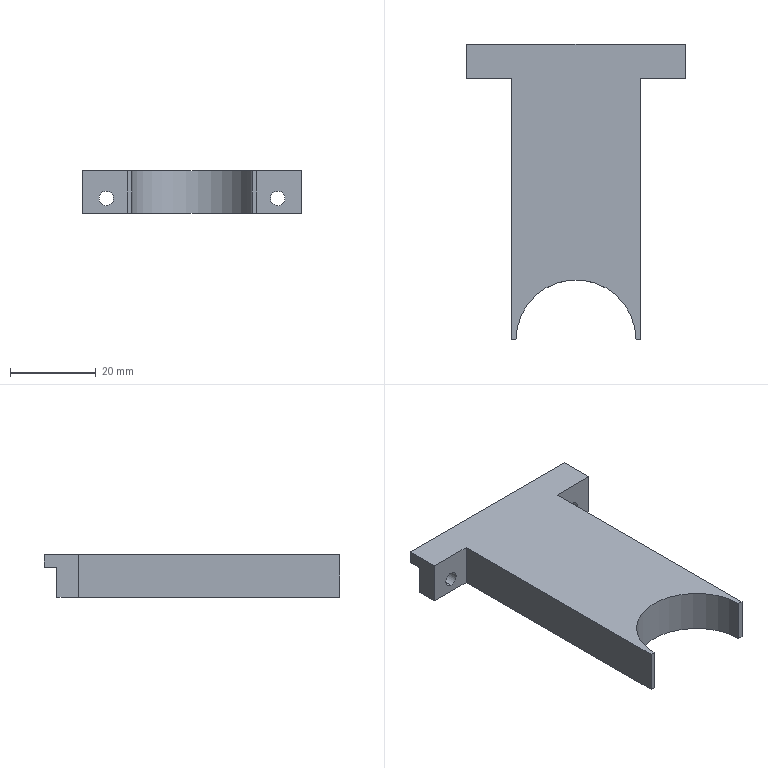Part | SolidWorks | features MoveFace 4, ICE 3, Cut 2, HoleWzd 2, Extrusion 1, MirrorPattern 1 | 1 solid | 22 faces | box 51 x 69 x 10 mm | volume 18117 mm3 | plane 13 | cylinder 5 | cone 4 | commonest cylinder face diameters 3.4 x4 28 x1
STEP:
#1=CARTESIAN_POINT('',(-20.,68.7,13.8));
#2=VERTEX_POINT('',#1);
#3=CARTESIAN_POINT('',(-20.,68.7,17.2));
#4=VERTEX_POINT('',#3);
#5=CARTESIAN_POINT('',(-20.,68.7,15.5));
#6=DIRECTION('',(0.,1.,0.));
#7=DIRECTION('',(0.,0.,1.));
#8=AXIS2_PLACEMENT_3D('',#5,#6,#7);
#9=CIRCLE('',#8,1.7);
#10=EDGE_CURVE('',#2,#4,#9,.T.);
#11=ORIENTED_EDGE('',*,*,#10,.F.);
#12=CARTESIAN_POINT('',(-20.,70.,12.5));
#13=VERTEX_POINT('',#12);
#14=CARTESIAN_POINT('',(-20.,70.,12.5));
#15=DIRECTION('',(0.,0.7071,-0.7071));
#16=VECTOR('',#15,1000.);
#17=LINE('',#14,#16);
#18=EDGE_CURVE('',#2,#13,#17,.T.);
#19=ORIENTED_EDGE('',*,*,#18,.T.);
#20=CARTESIAN_POINT('',(-20.,70.,18.5));
#21=VERTEX_POINT('',#20);
#22=CARTESIAN_POINT('',(-20.,70.,15.5));
#23=DIRECTION('',(0.,1.,0.));
#24=DIRECTION('',(0.,0.,1.));
#25=AXIS2_PLACEMENT_3D('',#22,#23,#24);
#26=CIRCLE('',#25,3.);
#27=EDGE_CURVE('',#13,#21,#26,.T.);
#28=ORIENTED_EDGE('',*,*,#27,.T.);
#29=CARTESIAN_POINT('',(-20.,70.,18.5));
#30=DIRECTION('',(0.,0.7071,0.7071));
#31=VECTOR('',#30,1000.);
#32=LINE('',#29,#31);
#33=EDGE_CURVE('',#4,#21,#32,.T.);
#34=ORIENTED_EDGE('',*,*,#33,.F.);
#35=EDGE_LOOP('',(#11,#19,#28,#34));
#36=FACE_OUTER_BOUND('',#35,.T.);
#37=CARTESIAN_POINT('',(-20.,70.,15.5));
#38=DIRECTION('',(0.,1.,0.));
#39=DIRECTION('',(0.,0.,1.));
#40=AXIS2_PLACEMENT_3D('',#37,#38,#39);
#41=CONICAL_SURFACE('',#40,3.,0.7854);
#42=ADVANCED_FACE('',(#36),#41,.F.);
#43=CARTESIAN_POINT('',(-20.,65.,13.8));
#44=VERTEX_POINT('',#43);
#45=CARTESIAN_POINT('',(-20.,65.,17.2));
#46=VERTEX_POINT('',#45);
#47=CARTESIAN_POINT('',(-20.,65.,15.5));
#48=DIRECTION('',(0.,1.,0.));
#49=DIRECTION('',(0.,0.,1.));
#50=AXIS2_PLACEMENT_3D('',#47,#48,#49);
#51=CIRCLE('',#50,1.7);
#52=EDGE_CURVE('',#44,#46,#51,.T.);
#53=ORIENTED_EDGE('',*,*,#52,.F.);
#54=CARTESIAN_POINT('',(-20.,70.,13.8));
#55=DIRECTION('',(0.,1.,0.));
#56=VECTOR('',#55,1000.);
#57=LINE('',#54,#56);
#58=EDGE_CURVE('',#44,#2,#57,.T.);
#59=ORIENTED_EDGE('',*,*,#58,.T.);
#60=ORIENTED_EDGE('',*,*,#10,.T.);
#61=CARTESIAN_POINT('',(-20.,70.,17.2));
#62=DIRECTION('',(0.,1.,0.));
#63=VECTOR('',#62,1000.);
#64=LINE('',#61,#63);
#65=EDGE_CURVE('',#46,#4,#64,.T.);
#66=ORIENTED_EDGE('',*,*,#65,.F.);
#67=EDGE_LOOP('',(#53,#59,#60,#66));
#68=FACE_OUTER_BOUND('',#67,.T.);
#69=CARTESIAN_POINT('',(-20.,70.,15.5));
#70=DIRECTION('',(0.,1.,0.));
#71=DIRECTION('',(0.,0.,1.));
#72=AXIS2_PLACEMENT_3D('',#69,#70,#71);
#73=CYLINDRICAL_SURFACE('',#72,1.7);
#74=ADVANCED_FACE('',(#68),#73,.F.);
#75=CARTESIAN_POINT('',(20.,68.7,13.8));
#76=VERTEX_POINT('',#75);
#77=CARTESIAN_POINT('',(20.,68.7,17.2));
#78=VERTEX_POINT('',#77);
#79=CARTESIAN_POINT('',(20.,68.7,15.5));
#80=DIRECTION('',(0.,1.,0.));
#81=DIRECTION('',(0.,0.,1.));
#82=AXIS2_PLACEMENT_3D('',#79,#80,#81);
#83=CIRCLE('',#82,1.7);
#84=EDGE_CURVE('',#76,#78,#83,.T.);
#85=ORIENTED_EDGE('',*,*,#84,.F.);
#86=CARTESIAN_POINT('',(20.,70.,12.5));
#87=VERTEX_POINT('',#86);
#88=CARTESIAN_POINT('',(20.,70.,12.5));
#89=DIRECTION('',(0.,0.7071,-0.7071));
#90=VECTOR('',#89,1000.);
#91=LINE('',#88,#90);
#92=EDGE_CURVE('',#76,#87,#91,.T.);
#93=ORIENTED_EDGE('',*,*,#92,.T.);
#94=CARTESIAN_POINT('',(20.,70.,18.5));
#95=VERTEX_POINT('',#94);
#96=CARTESIAN_POINT('',(20.,70.,15.5));
#97=DIRECTION('',(0.,1.,0.));
#98=DIRECTION('',(0.,0.,1.));
#99=AXIS2_PLACEMENT_3D('',#96,#97,#98);
#100=CIRCLE('',#99,3.);
#101=EDGE_CURVE('',#87,#95,#100,.T.);
#102=ORIENTED_EDGE('',*,*,#101,.T.);
#103=CARTESIAN_POINT('',(20.,70.,18.5));
#104=DIRECTION('',(0.,0.7071,0.7071));
#105=VECTOR('',#104,1000.);
#106=LINE('',#103,#105);
#107=EDGE_CURVE('',#78,#95,#106,.T.);
#108=ORIENTED_EDGE('',*,*,#107,.F.);
#109=EDGE_LOOP('',(#85,#93,#102,#108));
#110=FACE_OUTER_BOUND('',#109,.T.);
#111=CARTESIAN_POINT('',(20.,70.,15.5));
#112=DIRECTION('',(0.,1.,0.));
#113=DIRECTION('',(0.,0.,1.));
#114=AXIS2_PLACEMENT_3D('',#111,#112,#113);
#115=CONICAL_SURFACE('',#114,3.,0.7854);
#116=ADVANCED_FACE('',(#110),#115,.F.);
#117=CARTESIAN_POINT('',(20.,65.,17.2));
#118=VERTEX_POINT('',#117);
#119=CARTESIAN_POINT('',(20.,65.,13.8));
#120=VERTEX_POINT('',#119);
#121=CARTESIAN_POINT('',(20.,65.,15.5));
#122=DIRECTION('',(0.,-1.,0.));
#123=DIRECTION('',(0.,0.,-1.));
#124=AXIS2_PLACEMENT_3D('',#121,#122,#123);
#125=CIRCLE('',#124,1.7);
#126=EDGE_CURVE('',#118,#120,#125,.T.);
#127=ORIENTED_EDGE('',*,*,#126,.T.);
#128=CARTESIAN_POINT('',(20.,70.,13.8));
#129=DIRECTION('',(0.,1.,0.));
#130=VECTOR('',#129,1000.);
#131=LINE('',#128,#130);
#132=EDGE_CURVE('',#120,#76,#131,.T.);
#133=ORIENTED_EDGE('',*,*,#132,.T.);
#134=ORIENTED_EDGE('',*,*,#84,.T.);
#135=CARTESIAN_POINT('',(20.,70.,17.2));
#136=DIRECTION('',(0.,1.,0.));
#137=VECTOR('',#136,1000.);
#138=LINE('',#135,#137);
#139=EDGE_CURVE('',#118,#78,#138,.T.);
#140=ORIENTED_EDGE('',*,*,#139,.F.);
#141=EDGE_LOOP('',(#127,#133,#134,#140));
#142=FACE_OUTER_BOUND('',#141,.T.);
#143=CARTESIAN_POINT('',(20.,70.,15.5));
#144=DIRECTION('',(0.,1.,0.));
#145=DIRECTION('',(0.,0.,1.));
#146=AXIS2_PLACEMENT_3D('',#143,#144,#145);
#147=CYLINDRICAL_SURFACE('',#146,1.7);
#148=ADVANCED_FACE('',(#142),#147,.F.);
#149=CARTESIAN_POINT('',(-20.,70.,15.5));
#150=DIRECTION('',(0.,1.,0.));
#151=DIRECTION('',(0.,0.,1.));
#152=AXIS2_PLACEMENT_3D('',#149,#150,#151);
#153=CIRCLE('',#152,3.);
#154=EDGE_CURVE('',#21,#13,#153,.T.);
#155=ORIENTED_EDGE('',*,*,#154,.F.);
#156=ORIENTED_EDGE('',*,*,#27,.F.);
#157=EDGE_LOOP('',(#155,#156));
#158=FACE_BOUND('',#157,.T.);
#159=CARTESIAN_POINT('',(20.,70.,15.5));
#160=DIRECTION('',(0.,1.,0.));
#161=DIRECTION('',(0.,0.,1.));
#162=AXIS2_PLACEMENT_3D('',#159,#160,#161);
#163=CIRCLE('',#162,3.);
#164=EDGE_CURVE('',#95,#87,#163,.T.);
#165=ORIENTED_EDGE('',*,*,#164,.F.);
#166=ORIENTED_EDGE('',*,*,#101,.F.);
#167=EDGE_LOOP('',(#165,#166));
#168=FACE_BOUND('',#167,.T.);
#169=CARTESIAN_POINT('',(25.5,70.,19.));
#170=VERTEX_POINT('',#169);
#171=CARTESIAN_POINT('',(-25.5,70.,19.));
#172=VERTEX_POINT('',#171);
#173=CARTESIAN_POINT('',(-25.5,70.,19.));
#174=DIRECTION('',(-1.,0.,0.));
#175=VECTOR('',#174,1000.);
#176=LINE('',#173,#175);
#177=EDGE_CURVE('',#170,#172,#176,.T.);
#178=ORIENTED_EDGE('',*,*,#177,.F.);
#179=CARTESIAN_POINT('',(25.5,70.,12.));
#180=VERTEX_POINT('',#179);
#181=CARTESIAN_POINT('',(25.5,70.,12.));
#182=DIRECTION('',(0.,0.,-1.));
#183=VECTOR('',#182,1000.);
#184=LINE('',#181,#183);
#185=EDGE_CURVE('',#170,#180,#184,.T.);
#186=ORIENTED_EDGE('',*,*,#185,.T.);
#187=CARTESIAN_POINT('',(-25.5,70.,12.));
#188=VERTEX_POINT('',#187);
#189=CARTESIAN_POINT('',(-25.5,70.,12.));
#190=DIRECTION('',(-1.,0.,0.));
#191=VECTOR('',#190,1000.);
#192=LINE('',#189,#191);
#193=EDGE_CURVE('',#180,#188,#192,.T.);
#194=ORIENTED_EDGE('',*,*,#193,.T.);
#195=CARTESIAN_POINT('',(-25.5,70.,18.));
#196=DIRECTION('',(0.,0.,1.));
#197=VECTOR('',#196,1000.);
#198=LINE('',#195,#197);
#199=EDGE_CURVE('',#188,#172,#198,.T.);
#200=ORIENTED_EDGE('',*,*,#199,.T.);
#201=EDGE_LOOP('',(#178,#186,#194,#200));
#202=FACE_OUTER_BOUND('',#201,.T.);
#203=CARTESIAN_POINT('',(0.,70.,0.));
#204=DIRECTION('',(0.,-1.,0.));
#205=DIRECTION('',(0.,0.,-1.));
#206=AXIS2_PLACEMENT_3D('',#203,#204,#205);
#207=PLANE('',#206);
#208=ADVANCED_FACE('',(#158,#168,#202),#207,.F.);
#209=CARTESIAN_POINT('',(-15.,65.,12.));
#210=VERTEX_POINT('',#209);
#211=CARTESIAN_POINT('',(-15.,65.,22.));
#212=VERTEX_POINT('',#211);
#213=CARTESIAN_POINT('',(-15.,65.,15.));
#214=DIRECTION('',(0.,0.,1.));
#215=VECTOR('',#214,1000.);
#216=LINE('',#213,#215);
#217=EDGE_CURVE('',#210,#212,#216,.T.);
#218=ORIENTED_EDGE('',*,*,#217,.F.);
#219=CARTESIAN_POINT('',(-15.,4.,12.));
#220=VERTEX_POINT('',#219);
#221=CARTESIAN_POINT('',(-15.,0.,12.));
#222=DIRECTION('',(0.,-1.,0.));
#223=VECTOR('',#222,1000.);
#224=LINE('',#221,#223);
#225=EDGE_CURVE('',#210,#220,#224,.T.);
#226=ORIENTED_EDGE('',*,*,#225,.T.);
#227=CARTESIAN_POINT('',(-15.,4.,22.));
#228=VERTEX_POINT('',#227);
#229=CARTESIAN_POINT('',(-15.,4.,15.));
#230=DIRECTION('',(0.,0.,-1.));
#231=VECTOR('',#230,1000.);
#232=LINE('',#229,#231);
#233=EDGE_CURVE('',#228,#220,#232,.T.);
#234=ORIENTED_EDGE('',*,*,#233,.F.);
#235=CARTESIAN_POINT('',(-15.,0.,22.));
#236=DIRECTION('',(0.,-1.,0.));
#237=VECTOR('',#236,1000.);
#238=LINE('',#235,#237);
#239=EDGE_CURVE('',#212,#228,#238,.T.);
#240=ORIENTED_EDGE('',*,*,#239,.F.);
#241=EDGE_LOOP('',(#218,#226,#234,#240));
#242=FACE_OUTER_BOUND('',#241,.T.);
#243=CARTESIAN_POINT('',(-15.,0.,15.));
#244=DIRECTION('',(1.,0.,0.));
#245=DIRECTION('',(0.,0.,-1.));
#246=AXIS2_PLACEMENT_3D('',#243,#244,#245);
#247=PLANE('',#246);
#248=ADVANCED_FACE('',(#242),#247,.F.);
#249=ORIENTED_EDGE('',*,*,#233,.T.);
#250=CARTESIAN_POINT('',(-14.,4.,12.));
#251=VERTEX_POINT('',#250);
#252=CARTESIAN_POINT('',(-25.5,4.,12.));
#253=DIRECTION('',(1.,0.,0.));
#254=VECTOR('',#253,1000.);
#255=LINE('',#252,#254);
#256=EDGE_CURVE('',#220,#251,#255,.T.);
#257=ORIENTED_EDGE('',*,*,#256,.T.);
#258=CARTESIAN_POINT('',(-14.,4.,22.));
#259=VERTEX_POINT('',#258);
#260=CARTESIAN_POINT('',(-14.,4.,15.));
#261=DIRECTION('',(0.,0.,-1.));
#262=VECTOR('',#261,1000.);
#263=LINE('',#260,#262);
#264=EDGE_CURVE('',#259,#251,#263,.T.);
#265=ORIENTED_EDGE('',*,*,#264,.F.);
#266=CARTESIAN_POINT('',(-14.,4.,22.));
#267=DIRECTION('',(1.,0.,0.));
#268=VECTOR('',#267,1000.);
#269=LINE('',#266,#268);
#270=EDGE_CURVE('',#228,#259,#269,.T.);
#271=ORIENTED_EDGE('',*,*,#270,.F.);
#272=EDGE_LOOP('',(#249,#257,#265,#271));
#273=FACE_OUTER_BOUND('',#272,.T.);
#274=CARTESIAN_POINT('',(-14.,4.,15.));
#275=DIRECTION('',(0.,1.,0.));
#276=DIRECTION('',(0.,0.,1.));
#277=AXIS2_PLACEMENT_3D('',#274,#275,#276);
#278=PLANE('',#277);
#279=ADVANCED_FACE('',(#273),#278,.F.);
#280=ORIENTED_EDGE('',*,*,#264,.T.);
#281=CARTESIAN_POINT('',(14.,4.,12.));
#282=VERTEX_POINT('',#281);
#283=CARTESIAN_POINT('',(0.,4.,12.));
#284=DIRECTION('',(0.,0.,-1.));
#285=DIRECTION('',(1.,0.,0.));
#286=AXIS2_PLACEMENT_3D('',#283,#284,#285);
#287=CIRCLE('',#286,14.);
#288=EDGE_CURVE('',#251,#282,#287,.T.);
#289=ORIENTED_EDGE('',*,*,#288,.T.);
#290=CARTESIAN_POINT('',(14.,4.,22.));
#291=VERTEX_POINT('',#290);
#292=CARTESIAN_POINT('',(14.,4.,15.));
#293=DIRECTION('',(0.,0.,-1.));
#294=VECTOR('',#293,1000.);
#295=LINE('',#292,#294);
#296=EDGE_CURVE('',#291,#282,#295,.T.);
#297=ORIENTED_EDGE('',*,*,#296,.F.);
#298=CARTESIAN_POINT('',(0.,4.,22.));
#299=DIRECTION('',(0.,0.,-1.));
#300=DIRECTION('',(1.,0.,0.));
#301=AXIS2_PLACEMENT_3D('',#298,#299,#300);
#302=CIRCLE('',#301,14.);
#303=EDGE_CURVE('',#259,#291,#302,.T.);
#304=ORIENTED_EDGE('',*,*,#303,.F.);
#305=EDGE_LOOP('',(#280,#289,#297,#304));
#306=FACE_OUTER_BOUND('',#305,.T.);
#307=CARTESIAN_POINT('',(0.,4.,15.));
#308=DIRECTION('',(0.,0.,-1.));
#309=DIRECTION('',(-1.,0.,0.));
#310=AXIS2_PLACEMENT_3D('',#307,#308,#309);
#311=CYLINDRICAL_SURFACE('',#310,14.);
#312=ADVANCED_FACE('',(#306),#311,.F.);
#313=ORIENTED_EDGE('',*,*,#296,.T.);
#314=CARTESIAN_POINT('',(15.,4.,12.));
#315=VERTEX_POINT('',#314);
#316=CARTESIAN_POINT('',(-25.5,4.,12.));
#317=DIRECTION('',(1.,0.,0.));
#318=VECTOR('',#317,1000.);
#319=LINE('',#316,#318);
#320=EDGE_CURVE('',#282,#315,#319,.T.);
#321=ORIENTED_EDGE('',*,*,#320,.T.);
#322=CARTESIAN_POINT('',(15.,4.,22.));
#323=VERTEX_POINT('',#322);
#324=CARTESIAN_POINT('',(15.,4.,15.));
#325=DIRECTION('',(0.,0.,-1.));
#326=VECTOR('',#325,1000.);
#327=LINE('',#324,#326);
#328=EDGE_CURVE('',#323,#315,#327,.T.);
#329=ORIENTED_EDGE('',*,*,#328,.F.);
#330=CARTESIAN_POINT('',(14.,4.,22.));
#331=DIRECTION('',(1.,0.,0.));
#332=VECTOR('',#331,1000.);
#333=LINE('',#330,#332);
#334=EDGE_CURVE('',#291,#323,#333,.T.);
#335=ORIENTED_EDGE('',*,*,#334,.F.);
#336=EDGE_LOOP('',(#313,#321,#329,#335));
#337=FACE_OUTER_BOUND('',#336,.T.);
#338=CARTESIAN_POINT('',(14.,4.,15.));
#339=DIRECTION('',(0.,1.,0.));
#340=DIRECTION('',(0.,0.,1.));
#341=AXIS2_PLACEMENT_3D('',#338,#339,#340);
#342=PLANE('',#341);
#343=ADVANCED_FACE('',(#337),#342,.F.);
#344=ORIENTED_EDGE('',*,*,#328,.T.);
#345=CARTESIAN_POINT('',(15.,65.,12.));
#346=VERTEX_POINT('',#345);
#347=CARTESIAN_POINT('',(15.,0.,12.));
#348=DIRECTION('',(0.,1.,0.));
#349=VECTOR('',#348,1000.);
#350=LINE('',#347,#349);
#351=EDGE_CURVE('',#315,#346,#350,.T.);
#352=ORIENTED_EDGE('',*,*,#351,.T.);
#353=CARTESIAN_POINT('',(15.,65.,22.));
#354=VERTEX_POINT('',#353);
#355=CARTESIAN_POINT('',(15.,65.,15.));
#356=DIRECTION('',(0.,0.,1.));
#357=VECTOR('',#356,1000.);
#358=LINE('',#355,#357);
#359=EDGE_CURVE('',#346,#354,#358,.T.);
#360=ORIENTED_EDGE('',*,*,#359,.T.);
#361=CARTESIAN_POINT('',(15.,0.,22.));
#362=DIRECTION('',(0.,1.,0.));
#363=VECTOR('',#362,1000.);
#364=LINE('',#361,#363);
#365=EDGE_CURVE('',#323,#354,#364,.T.);
#366=ORIENTED_EDGE('',*,*,#365,.F.);
#367=EDGE_LOOP('',(#344,#352,#360,#366));
#368=FACE_OUTER_BOUND('',#367,.T.);
#369=CARTESIAN_POINT('',(15.,0.,15.));
#370=DIRECTION('',(-1.,0.,0.));
#371=DIRECTION('',(0.,0.,1.));
#372=AXIS2_PLACEMENT_3D('',#369,#370,#371);
#373=PLANE('',#372);
#374=ADVANCED_FACE('',(#368),#373,.F.);
#375=CARTESIAN_POINT('',(25.5,65.,22.));
#376=VERTEX_POINT('',#375);
#377=CARTESIAN_POINT('',(25.5,73.,22.));
#378=VERTEX_POINT('',#377);
#379=CARTESIAN_POINT('',(25.5,65.,22.));
#380=DIRECTION('',(0.,1.,0.));
#381=VECTOR('',#380,1000.);
#382=LINE('',#379,#381);
#383=EDGE_CURVE('',#376,#378,#382,.T.);
#384=ORIENTED_EDGE('',*,*,#383,.T.);
#385=CARTESIAN_POINT('',(-25.5,73.,22.));
#386=VERTEX_POINT('',#385);
#387=CARTESIAN_POINT('',(-25.5,73.,22.));
#388=DIRECTION('',(1.,0.,0.));
#389=VECTOR('',#388,1000.);
#390=LINE('',#387,#389);
#391=EDGE_CURVE('',#386,#378,#390,.T.);
#392=ORIENTED_EDGE('',*,*,#391,.F.);
#393=CARTESIAN_POINT('',(-25.5,65.,22.));
#394=VERTEX_POINT('',#393);
#395=CARTESIAN_POINT('',(-25.5,65.,22.));
#396=DIRECTION('',(0.,1.,0.));
#397=VECTOR('',#396,1000.);
#398=LINE('',#395,#397);
#399=EDGE_CURVE('',#394,#386,#398,.T.);
#400=ORIENTED_EDGE('',*,*,#399,.F.);
#401=CARTESIAN_POINT('',(-25.5,65.,22.));
#402=DIRECTION('',(1.,0.,0.));
#403=VECTOR('',#402,1000.);
#404=LINE('',#401,#403);
#405=EDGE_CURVE('',#394,#212,#404,.T.);
#406=ORIENTED_EDGE('',*,*,#405,.T.);
#407=ORIENTED_EDGE('',*,*,#239,.T.);
#408=ORIENTED_EDGE('',*,*,#270,.T.);
#409=ORIENTED_EDGE('',*,*,#303,.T.);
#410=ORIENTED_EDGE('',*,*,#334,.T.);
#411=ORIENTED_EDGE('',*,*,#365,.T.);
#412=CARTESIAN_POINT('',(25.5,65.,22.));
#413=DIRECTION('',(-1.,0.,0.));
#414=VECTOR('',#413,1000.);
#415=LINE('',#412,#414);
#416=EDGE_CURVE('',#376,#354,#415,.T.);
#417=ORIENTED_EDGE('',*,*,#416,.F.);
#418=EDGE_LOOP('',(#384,#392,#400,#406,#407,#408,#409,#410,#411,#417));
#419=FACE_OUTER_BOUND('',#418,.T.);
#420=CARTESIAN_POINT('',(0.,0.,22.));
#421=DIRECTION('',(0.,0.,1.));
#422=DIRECTION('',(1.,0.,0.));
#423=AXIS2_PLACEMENT_3D('',#420,#421,#422);
#424=PLANE('',#423);
#425=ADVANCED_FACE('',(#419),#424,.T.);
#426=CARTESIAN_POINT('',(-20.,65.,15.5));
#427=DIRECTION('',(0.,1.,0.));
#428=DIRECTION('',(0.,0.,1.));
#429=AXIS2_PLACEMENT_3D('',#426,#427,#428);
#430=CIRCLE('',#429,1.7);
#431=EDGE_CURVE('',#46,#44,#430,.T.);
#432=ORIENTED_EDGE('',*,*,#431,.T.);
#433=ORIENTED_EDGE('',*,*,#52,.T.);
#434=EDGE_LOOP('',(#432,#433));
#435=FACE_BOUND('',#434,.T.);
#436=CARTESIAN_POINT('',(-25.5,65.,12.));
#437=VERTEX_POINT('',#436);
#438=CARTESIAN_POINT('',(-25.5,65.,15.));
#439=DIRECTION('',(0.,0.,1.));
#440=VECTOR('',#439,1000.);
#441=LINE('',#438,#440);
#442=EDGE_CURVE('',#437,#394,#441,.T.);
#443=ORIENTED_EDGE('',*,*,#442,.F.);
#444=CARTESIAN_POINT('',(-25.5,65.,12.));
#445=DIRECTION('',(1.,0.,0.));
#446=VECTOR('',#445,1000.);
#447=LINE('',#444,#446);
#448=EDGE_CURVE('',#437,#210,#447,.T.);
#449=ORIENTED_EDGE('',*,*,#448,.T.);
#450=ORIENTED_EDGE('',*,*,#217,.T.);
#451=ORIENTED_EDGE('',*,*,#405,.F.);
#452=EDGE_LOOP('',(#443,#449,#450,#451));
#453=FACE_OUTER_BOUND('',#452,.T.);
#454=CARTESIAN_POINT('',(-25.5,65.,15.));
#455=DIRECTION('',(0.,1.,0.));
#456=DIRECTION('',(0.,0.,1.));
#457=AXIS2_PLACEMENT_3D('',#454,#455,#456);
#458=PLANE('',#457);
#459=ADVANCED_FACE('',(#435,#453),#458,.F.);
#460=CARTESIAN_POINT('',(-25.5,70.,12.));
#461=DIRECTION('',(0.,-1.,0.));
#462=VECTOR('',#461,1000.);
#463=LINE('',#460,#462);
#464=EDGE_CURVE('',#188,#437,#463,.T.);
#465=ORIENTED_EDGE('',*,*,#464,.T.);
#466=ORIENTED_EDGE('',*,*,#442,.T.);
#467=ORIENTED_EDGE('',*,*,#399,.T.);
#468=CARTESIAN_POINT('',(-25.5,73.,19.));
#469=VERTEX_POINT('',#468);
#470=CARTESIAN_POINT('',(-25.5,73.,19.));
#471=DIRECTION('',(0.,0.,1.));
#472=VECTOR('',#471,1000.);
#473=LINE('',#470,#472);
#474=EDGE_CURVE('',#469,#386,#473,.T.);
#475=ORIENTED_EDGE('',*,*,#474,.F.);
#476=CARTESIAN_POINT('',(-25.5,73.,19.));
#477=DIRECTION('',(0.,-1.,0.));
#478=VECTOR('',#477,1000.);
#479=LINE('',#476,#478);
#480=EDGE_CURVE('',#469,#172,#479,.T.);
#481=ORIENTED_EDGE('',*,*,#480,.T.);
#482=ORIENTED_EDGE('',*,*,#199,.F.);
#483=EDGE_LOOP('',(#465,#466,#467,#475,#481,#482));
#484=FACE_OUTER_BOUND('',#483,.T.);
#485=CARTESIAN_POINT('',(-25.5,0.,0.));
#486=DIRECTION('',(1.,0.,0.));
#487=DIRECTION('',(0.,0.,-1.));
#488=AXIS2_PLACEMENT_3D('',#485,#486,#487);
#489=PLANE('',#488);
#490=ADVANCED_FACE('',(#484),#489,.F.);
#491=ORIENTED_EDGE('',*,*,#126,.F.);
#492=CARTESIAN_POINT('',(20.,65.,15.5));
#493=DIRECTION('',(0.,-1.,0.));
#494=DIRECTION('',(0.,0.,-1.));
#495=AXIS2_PLACEMENT_3D('',#492,#493,#494);
#496=CIRCLE('',#495,1.7);
#497=EDGE_CURVE('',#120,#118,#496,.T.);
#498=ORIENTED_EDGE('',*,*,#497,.F.);
#499=EDGE_LOOP('',(#491,#498));
#500=FACE_BOUND('',#499,.T.);
#501=CARTESIAN_POINT('',(25.5,65.,12.));
#502=VERTEX_POINT('',#501);
#503=CARTESIAN_POINT('',(25.5,65.,12.));
#504=DIRECTION('',(-1.,0.,0.));
#505=VECTOR('',#504,1000.);
#506=LINE('',#503,#505);
#507=EDGE_CURVE('',#502,#346,#506,.T.);
#508=ORIENTED_EDGE('',*,*,#507,.F.);
#509=CARTESIAN_POINT('',(25.5,65.,15.));
#510=DIRECTION('',(0.,0.,1.));
#511=VECTOR('',#510,1000.);
#512=LINE('',#509,#511);
#513=EDGE_CURVE('',#502,#376,#512,.T.);
#514=ORIENTED_EDGE('',*,*,#513,.T.);
#515=ORIENTED_EDGE('',*,*,#416,.T.);
#516=ORIENTED_EDGE('',*,*,#359,.F.);
#517=EDGE_LOOP('',(#508,#514,#515,#516));
#518=FACE_OUTER_BOUND('',#517,.T.);
#519=CARTESIAN_POINT('',(25.5,65.,15.));
#520=DIRECTION('',(0.,-1.,0.));
#521=DIRECTION('',(0.,0.,-1.));
#522=AXIS2_PLACEMENT_3D('',#519,#520,#521);
#523=PLANE('',#522);
#524=ADVANCED_FACE('',(#500,#518),#523,.T.);
#525=ORIENTED_EDGE('',*,*,#513,.F.);
#526=CARTESIAN_POINT('',(25.5,70.,12.));
#527=DIRECTION('',(0.,-1.,0.));
#528=VECTOR('',#527,1000.);
#529=LINE('',#526,#528);
#530=EDGE_CURVE('',#180,#502,#529,.T.);
#531=ORIENTED_EDGE('',*,*,#530,.F.);
#532=ORIENTED_EDGE('',*,*,#185,.F.);
#533=CARTESIAN_POINT('',(25.5,73.,19.));
#534=VERTEX_POINT('',#533);
#535=CARTESIAN_POINT('',(25.5,73.,19.));
#536=DIRECTION('',(0.,-1.,0.));
#537=VECTOR('',#536,1000.);
#538=LINE('',#535,#537);
#539=EDGE_CURVE('',#534,#170,#538,.T.);
#540=ORIENTED_EDGE('',*,*,#539,.F.);
#541=CARTESIAN_POINT('',(25.5,73.,22.));
#542=DIRECTION('',(0.,0.,-1.));
#543=VECTOR('',#542,1000.);
#544=LINE('',#541,#543);
#545=EDGE_CURVE('',#378,#534,#544,.T.);
#546=ORIENTED_EDGE('',*,*,#545,.F.);
#547=ORIENTED_EDGE('',*,*,#383,.F.);
#548=EDGE_LOOP('',(#525,#531,#532,#540,#546,#547));
#549=FACE_OUTER_BOUND('',#548,.T.);
#550=CARTESIAN_POINT('',(25.5,0.,0.));
#551=DIRECTION('',(-1.,0.,0.));
#552=DIRECTION('',(0.,0.,-1.));
#553=AXIS2_PLACEMENT_3D('',#550,#551,#552);
#554=PLANE('',#553);
#555=ADVANCED_FACE('',(#549),#554,.F.);
#556=ORIENTED_EDGE('',*,*,#530,.T.);
#557=ORIENTED_EDGE('',*,*,#507,.T.);
#558=ORIENTED_EDGE('',*,*,#351,.F.);
#559=ORIENTED_EDGE('',*,*,#320,.F.);
#560=ORIENTED_EDGE('',*,*,#288,.F.);
#561=ORIENTED_EDGE('',*,*,#256,.F.);
#562=ORIENTED_EDGE('',*,*,#225,.F.);
#563=ORIENTED_EDGE('',*,*,#448,.F.);
#564=ORIENTED_EDGE('',*,*,#464,.F.);
#565=ORIENTED_EDGE('',*,*,#193,.F.);
#566=EDGE_LOOP('',(#556,#557,#558,#559,#560,#561,#562,#563,#564,#565));
#567=FACE_OUTER_BOUND('',#566,.T.);
#568=CARTESIAN_POINT('',(-25.5,70.,12.));
#569=DIRECTION('',(0.,0.,1.));
#570=DIRECTION('',(1.,0.,0.));
#571=AXIS2_PLACEMENT_3D('',#568,#569,#570);
#572=PLANE('',#571);
#573=ADVANCED_FACE('',(#567),#572,.F.);
#574=ORIENTED_EDGE('',*,*,#177,.T.);
#575=ORIENTED_EDGE('',*,*,#480,.F.);
#576=CARTESIAN_POINT('',(-25.5,73.,19.));
#577=DIRECTION('',(-1.,0.,0.));
#578=VECTOR('',#577,1000.);
#579=LINE('',#576,#578);
#580=EDGE_CURVE('',#534,#469,#579,.T.);
#581=ORIENTED_EDGE('',*,*,#580,.F.);
#582=ORIENTED_EDGE('',*,*,#539,.T.);
#583=EDGE_LOOP('',(#574,#575,#581,#582));
#584=FACE_OUTER_BOUND('',#583,.T.);
#585=CARTESIAN_POINT('',(-25.5,73.,19.));
#586=DIRECTION('',(0.,0.,1.));
#587=DIRECTION('',(1.,0.,0.));
#588=AXIS2_PLACEMENT_3D('',#585,#586,#587);
#589=PLANE('',#588);
#590=ADVANCED_FACE('',(#584),#589,.F.);
#591=ORIENTED_EDGE('',*,*,#391,.T.);
#592=ORIENTED_EDGE('',*,*,#545,.T.);
#593=ORIENTED_EDGE('',*,*,#580,.T.);
#594=ORIENTED_EDGE('',*,*,#474,.T.);
#595=EDGE_LOOP('',(#591,#592,#593,#594));
#596=FACE_OUTER_BOUND('',#595,.T.);
#597=CARTESIAN_POINT('',(0.,73.,0.));
#598=DIRECTION('',(0.,1.,0.));
#599=DIRECTION('',(0.,0.,1.));
#600=AXIS2_PLACEMENT_3D('',#597,#598,#599);
#601=PLANE('',#600);
#602=ADVANCED_FACE('',(#596),#601,.T.);
#603=ORIENTED_EDGE('',*,*,#132,.F.);
#604=ORIENTED_EDGE('',*,*,#497,.T.);
#605=ORIENTED_EDGE('',*,*,#139,.T.);
#606=CARTESIAN_POINT('',(20.,68.7,15.5));
#607=DIRECTION('',(0.,1.,0.));
#608=DIRECTION('',(0.,0.,1.));
#609=AXIS2_PLACEMENT_3D('',#606,#607,#608);
#610=CIRCLE('',#609,1.7);
#611=EDGE_CURVE('',#78,#76,#610,.T.);
#612=ORIENTED_EDGE('',*,*,#611,.T.);
#613=EDGE_LOOP('',(#603,#604,#605,#612));
#614=FACE_OUTER_BOUND('',#613,.T.);
#615=CARTESIAN_POINT('',(20.,70.,15.5));
#616=DIRECTION('',(0.,1.,0.));
#617=DIRECTION('',(0.,0.,1.));
#618=AXIS2_PLACEMENT_3D('',#615,#616,#617);
#619=CYLINDRICAL_SURFACE('',#618,1.7);
#620=ADVANCED_FACE('',(#614),#619,.F.);
#621=ORIENTED_EDGE('',*,*,#92,.F.);
#622=ORIENTED_EDGE('',*,*,#611,.F.);
#623=ORIENTED_EDGE('',*,*,#107,.T.);
#624=ORIENTED_EDGE('',*,*,#164,.T.);
#625=EDGE_LOOP('',(#621,#622,#623,#624));
#626=FACE_OUTER_BOUND('',#625,.T.);
#627=CARTESIAN_POINT('',(20.,70.,15.5));
#628=DIRECTION('',(0.,1.,0.));
#629=DIRECTION('',(0.,0.,1.));
#630=AXIS2_PLACEMENT_3D('',#627,#628,#629);
#631=CONICAL_SURFACE('',#630,3.,0.7854);
#632=ADVANCED_FACE('',(#626),#631,.F.);
#633=ORIENTED_EDGE('',*,*,#58,.F.);
#634=ORIENTED_EDGE('',*,*,#431,.F.);
#635=ORIENTED_EDGE('',*,*,#65,.T.);
#636=CARTESIAN_POINT('',(-20.,68.7,15.5));
#637=DIRECTION('',(0.,1.,0.));
#638=DIRECTION('',(0.,0.,1.));
#639=AXIS2_PLACEMENT_3D('',#636,#637,#638);
#640=CIRCLE('',#639,1.7);
#641=EDGE_CURVE('',#4,#2,#640,.T.);
#642=ORIENTED_EDGE('',*,*,#641,.T.);
#643=EDGE_LOOP('',(#633,#634,#635,#642));
#644=FACE_OUTER_BOUND('',#643,.T.);
#645=CARTESIAN_POINT('',(-20.,70.,15.5));
#646=DIRECTION('',(0.,1.,0.));
#647=DIRECTION('',(0.,0.,1.));
#648=AXIS2_PLACEMENT_3D('',#645,#646,#647);
#649=CYLINDRICAL_SURFACE('',#648,1.7);
#650=ADVANCED_FACE('',(#644),#649,.F.);
#651=ORIENTED_EDGE('',*,*,#18,.F.);
#652=ORIENTED_EDGE('',*,*,#641,.F.);
#653=ORIENTED_EDGE('',*,*,#33,.T.);
#654=ORIENTED_EDGE('',*,*,#154,.T.);
#655=EDGE_LOOP('',(#651,#652,#653,#654));
#656=FACE_OUTER_BOUND('',#655,.T.);
#657=CARTESIAN_POINT('',(-20.,70.,15.5));
#658=DIRECTION('',(0.,1.,0.));
#659=DIRECTION('',(0.,0.,1.));
#660=AXIS2_PLACEMENT_3D('',#657,#658,#659);
#661=CONICAL_SURFACE('',#660,3.,0.7854);
#662=ADVANCED_FACE('',(#656),#661,.F.);
#663=CLOSED_SHELL('',(#42,#74,#116,#148,#208,#248,#279,#312,#343,#374,#425,#459,#490,#524,#555,#573,#590,#602,#620,#632,#650,#662));
#664=MANIFOLD_SOLID_BREP('',#663);
#665=CARTESIAN_POINT('',(0.,0.,0.));
#666=DIRECTION('',(0.,0.,1.));
#667=DIRECTION('',(1.,0.,0.));
#668=AXIS2_PLACEMENT_3D('',#665,#666,#667);
#669=(LENGTH_UNIT()NAMED_UNIT(*)SI_UNIT(.MILLI.,.METRE.));
#670=UNCERTAINTY_MEASURE_WITH_UNIT(LENGTH_MEASURE(0.00001),#669,'','');
#671=(NAMED_UNIT(*)PLANE_ANGLE_UNIT()SI_UNIT($,.RADIAN.));
#672=(NAMED_UNIT(*)SI_UNIT($,.STERADIAN.)SOLID_ANGLE_UNIT());
#673=(GEOMETRIC_REPRESENTATION_CONTEXT(3)GLOBAL_UNCERTAINTY_ASSIGNED_CONTEXT((#670))GLOBAL_UNIT_ASSIGNED_CONTEXT((#669,#671,#672))REPRESENTATION_CONTEXT('',''));
#674=ADVANCED_BREP_SHAPE_REPRESENTATION('',(#664,#668),#673);